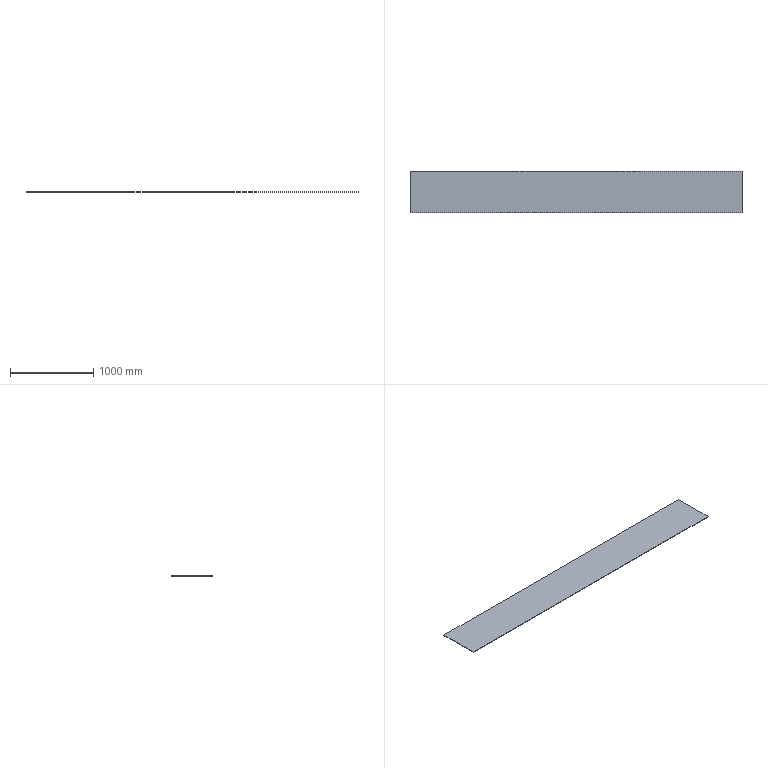Part | SolidWorks | features FlatPattern 1, SMBaseFlange 1, SheetMetal 1 | 1 solid | 6 faces | box 4000 x 500 x 6 mm | volume 12000000 mm3 | plane 6
STEP:
#1=CARTESIAN_POINT('',(-2000.,250.,0.));
#2=VERTEX_POINT('',#1);
#3=CARTESIAN_POINT('',(-2000.,-250.,0.));
#4=VERTEX_POINT('',#3);
#5=CARTESIAN_POINT('',(-2000.,-250.,0.));
#6=DIRECTION('',(0.,-1.,0.));
#7=VECTOR('',#6,1000.);
#8=LINE('',#5,#7);
#9=EDGE_CURVE('',#2,#4,#8,.T.);
#10=ORIENTED_EDGE('',*,*,#9,.F.);
#11=CARTESIAN_POINT('',(-2000.,250.,-6.));
#12=VERTEX_POINT('',#11);
#13=CARTESIAN_POINT('',(-2000.,250.,-6.));
#14=DIRECTION('',(0.,0.,1.));
#15=VECTOR('',#14,1000.);
#16=LINE('',#13,#15);
#17=EDGE_CURVE('',#12,#2,#16,.T.);
#18=ORIENTED_EDGE('',*,*,#17,.F.);
#19=CARTESIAN_POINT('',(-2000.,-250.,-6.));
#20=VERTEX_POINT('',#19);
#21=CARTESIAN_POINT('',(-2000.,-250.,-6.));
#22=DIRECTION('',(0.,-1.,0.));
#23=VECTOR('',#22,1000.);
#24=LINE('',#21,#23);
#25=EDGE_CURVE('',#12,#20,#24,.T.);
#26=ORIENTED_EDGE('',*,*,#25,.T.);
#27=CARTESIAN_POINT('',(-2000.,-250.,-6.));
#28=DIRECTION('',(0.,0.,1.));
#29=VECTOR('',#28,1000.);
#30=LINE('',#27,#29);
#31=EDGE_CURVE('',#20,#4,#30,.T.);
#32=ORIENTED_EDGE('',*,*,#31,.T.);
#33=EDGE_LOOP('',(#10,#18,#26,#32));
#34=FACE_OUTER_BOUND('',#33,.T.);
#35=CARTESIAN_POINT('',(-2000.,-250.,-6.));
#36=DIRECTION('',(-1.,0.,0.));
#37=DIRECTION('',(0.,-1.,0.));
#38=AXIS2_PLACEMENT_3D('',#35,#36,#37);
#39=PLANE('',#38);
#40=ADVANCED_FACE('',(#34),#39,.T.);
#41=CARTESIAN_POINT('',(2000.,250.,0.));
#42=VERTEX_POINT('',#41);
#43=CARTESIAN_POINT('',(2000.,250.,0.));
#44=DIRECTION('',(-1.,0.,0.));
#45=VECTOR('',#44,1000.);
#46=LINE('',#43,#45);
#47=EDGE_CURVE('',#42,#2,#46,.T.);
#48=ORIENTED_EDGE('',*,*,#47,.F.);
#49=CARTESIAN_POINT('',(2000.,250.,-6.));
#50=VERTEX_POINT('',#49);
#51=CARTESIAN_POINT('',(2000.,250.,-6.));
#52=DIRECTION('',(0.,0.,1.));
#53=VECTOR('',#52,1000.);
#54=LINE('',#51,#53);
#55=EDGE_CURVE('',#50,#42,#54,.T.);
#56=ORIENTED_EDGE('',*,*,#55,.F.);
#57=CARTESIAN_POINT('',(2000.,250.,-6.));
#58=DIRECTION('',(-1.,0.,0.));
#59=VECTOR('',#58,1000.);
#60=LINE('',#57,#59);
#61=EDGE_CURVE('',#50,#12,#60,.T.);
#62=ORIENTED_EDGE('',*,*,#61,.T.);
#63=ORIENTED_EDGE('',*,*,#17,.T.);
#64=EDGE_LOOP('',(#48,#56,#62,#63));
#65=FACE_OUTER_BOUND('',#64,.T.);
#66=CARTESIAN_POINT('',(2000.,250.,-6.));
#67=DIRECTION('',(0.,1.,0.));
#68=DIRECTION('',(-1.,0.,0.));
#69=AXIS2_PLACEMENT_3D('',#66,#67,#68);
#70=PLANE('',#69);
#71=ADVANCED_FACE('',(#65),#70,.T.);
#72=CARTESIAN_POINT('',(2000.,-250.,0.));
#73=VERTEX_POINT('',#72);
#74=CARTESIAN_POINT('',(2000.,-250.,0.));
#75=DIRECTION('',(0.,1.,0.));
#76=VECTOR('',#75,1000.);
#77=LINE('',#74,#76);
#78=EDGE_CURVE('',#73,#42,#77,.T.);
#79=ORIENTED_EDGE('',*,*,#78,.F.);
#80=CARTESIAN_POINT('',(2000.,-250.,-6.));
#81=VERTEX_POINT('',#80);
#82=CARTESIAN_POINT('',(2000.,-250.,-6.));
#83=DIRECTION('',(0.,0.,1.));
#84=VECTOR('',#83,1000.);
#85=LINE('',#82,#84);
#86=EDGE_CURVE('',#81,#73,#85,.T.);
#87=ORIENTED_EDGE('',*,*,#86,.F.);
#88=CARTESIAN_POINT('',(2000.,-250.,-6.));
#89=DIRECTION('',(0.,1.,0.));
#90=VECTOR('',#89,1000.);
#91=LINE('',#88,#90);
#92=EDGE_CURVE('',#81,#50,#91,.T.);
#93=ORIENTED_EDGE('',*,*,#92,.T.);
#94=ORIENTED_EDGE('',*,*,#55,.T.);
#95=EDGE_LOOP('',(#79,#87,#93,#94));
#96=FACE_OUTER_BOUND('',#95,.T.);
#97=CARTESIAN_POINT('',(2000.,-250.,-6.));
#98=DIRECTION('',(1.,0.,0.));
#99=DIRECTION('',(0.,0.,-1.));
#100=AXIS2_PLACEMENT_3D('',#97,#98,#99);
#101=PLANE('',#100);
#102=ADVANCED_FACE('',(#96),#101,.T.);
#103=CARTESIAN_POINT('',(2000.,-250.,0.));
#104=DIRECTION('',(1.,0.,0.));
#105=VECTOR('',#104,1000.);
#106=LINE('',#103,#105);
#107=EDGE_CURVE('',#4,#73,#106,.T.);
#108=ORIENTED_EDGE('',*,*,#107,.F.);
#109=ORIENTED_EDGE('',*,*,#31,.F.);
#110=CARTESIAN_POINT('',(2000.,-250.,-6.));
#111=DIRECTION('',(1.,0.,0.));
#112=VECTOR('',#111,1000.);
#113=LINE('',#110,#112);
#114=EDGE_CURVE('',#20,#81,#113,.T.);
#115=ORIENTED_EDGE('',*,*,#114,.T.);
#116=ORIENTED_EDGE('',*,*,#86,.T.);
#117=EDGE_LOOP('',(#108,#109,#115,#116));
#118=FACE_OUTER_BOUND('',#117,.T.);
#119=CARTESIAN_POINT('',(2000.,-250.,-6.));
#120=DIRECTION('',(0.,-1.,0.));
#121=DIRECTION('',(1.,0.,0.));
#122=AXIS2_PLACEMENT_3D('',#119,#120,#121);
#123=PLANE('',#122);
#124=ADVANCED_FACE('',(#118),#123,.T.);
#125=ORIENTED_EDGE('',*,*,#25,.F.);
#126=ORIENTED_EDGE('',*,*,#61,.F.);
#127=ORIENTED_EDGE('',*,*,#92,.F.);
#128=ORIENTED_EDGE('',*,*,#114,.F.);
#129=EDGE_LOOP('',(#125,#126,#127,#128));
#130=FACE_OUTER_BOUND('',#129,.T.);
#131=CARTESIAN_POINT('',(0.,0.,-6.));
#132=DIRECTION('',(0.,0.,1.));
#133=DIRECTION('',(1.,0.,0.));
#134=AXIS2_PLACEMENT_3D('',#131,#132,#133);
#135=PLANE('',#134);
#136=ADVANCED_FACE('',(#130),#135,.F.);
#137=ORIENTED_EDGE('',*,*,#9,.T.);
#138=ORIENTED_EDGE('',*,*,#107,.T.);
#139=ORIENTED_EDGE('',*,*,#78,.T.);
#140=ORIENTED_EDGE('',*,*,#47,.T.);
#141=EDGE_LOOP('',(#137,#138,#139,#140));
#142=FACE_OUTER_BOUND('',#141,.T.);
#143=CARTESIAN_POINT('',(0.,0.,0.));
#144=DIRECTION('',(0.,0.,1.));
#145=DIRECTION('',(1.,0.,0.));
#146=AXIS2_PLACEMENT_3D('',#143,#144,#145);
#147=PLANE('',#146);
#148=ADVANCED_FACE('',(#142),#147,.T.);
#149=CLOSED_SHELL('',(#40,#71,#102,#124,#136,#148));
#150=MANIFOLD_SOLID_BREP('',#149);
#151=CARTESIAN_POINT('',(0.,0.,0.));
#152=DIRECTION('',(0.,0.,1.));
#153=DIRECTION('',(1.,0.,0.));
#154=AXIS2_PLACEMENT_3D('',#151,#152,#153);
#155=(LENGTH_UNIT()NAMED_UNIT(*)SI_UNIT(.MILLI.,.METRE.));
#156=UNCERTAINTY_MEASURE_WITH_UNIT(LENGTH_MEASURE(0.00001),#155,'','');
#157=(NAMED_UNIT(*)PLANE_ANGLE_UNIT()SI_UNIT($,.RADIAN.));
#158=(NAMED_UNIT(*)SI_UNIT($,.STERADIAN.)SOLID_ANGLE_UNIT());
#159=(GEOMETRIC_REPRESENTATION_CONTEXT(3)GLOBAL_UNCERTAINTY_ASSIGNED_CONTEXT((#156))GLOBAL_UNIT_ASSIGNED_CONTEXT((#155,#157,#158))REPRESENTATION_CONTEXT('',''));
#160=ADVANCED_BREP_SHAPE_REPRESENTATION('',(#150,#154),#159);